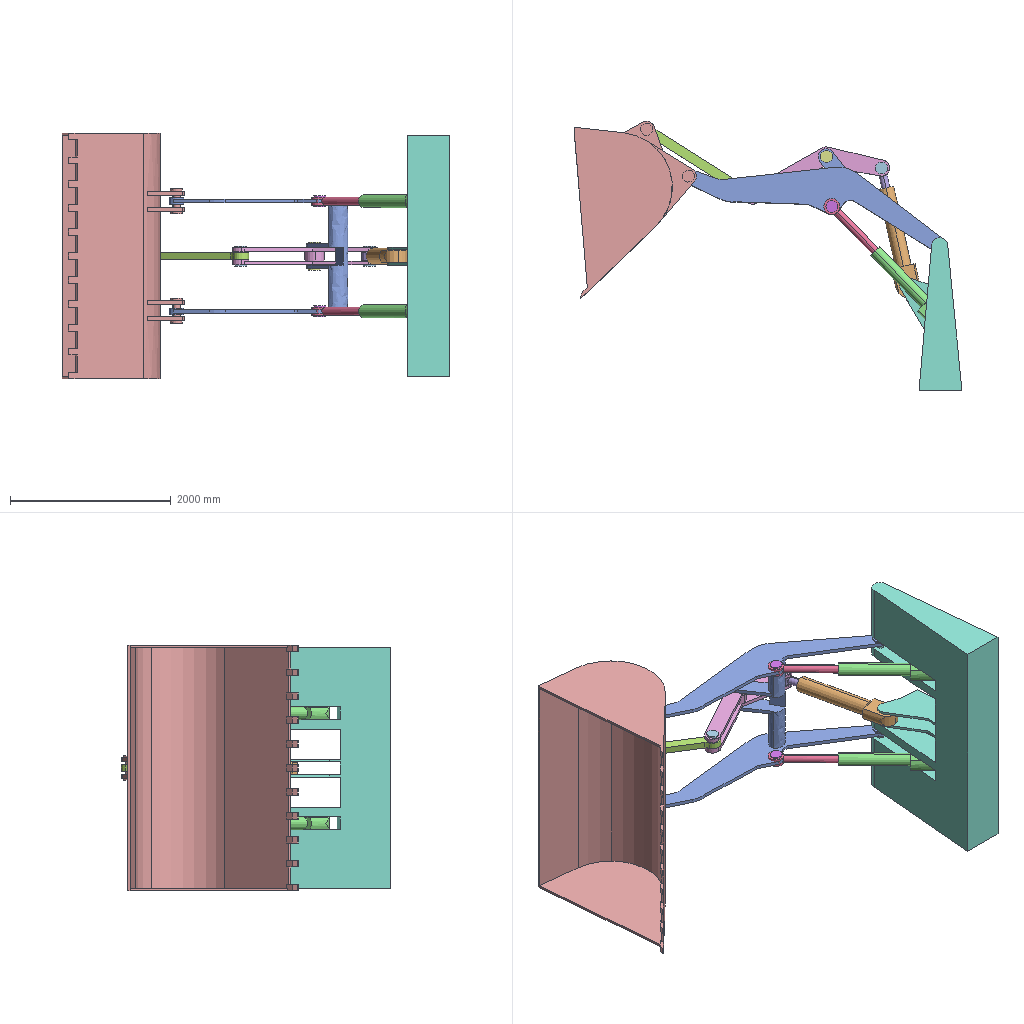Assembly | SolidWorks | 12 different items | 16 placed | box 4827 x 3349 x 3060 mm
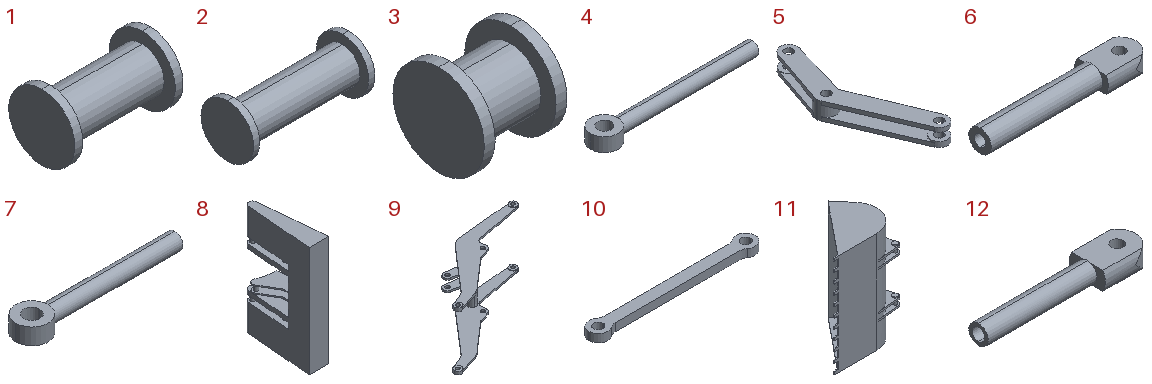Parts list (item | quantity | size | volume | features):
1 | x2 | 246 x 150 x 150 mm | 2285509 mm3 | features ICE 2, Extrusion 1
2 | x1 | 347 x 150 x 150 mm | 3078761 mm3 | features ICE 2, Extrusion 1
3 | x2 | 136 x 150 x 150 mm | 1421571 mm3 | features ICE 2, Extrusion 1
4 | x2 | 1182 x 200 x 100 mm | 10096773 mm3 | features Extrusion 1, ICE 1
5 | x1 | 614.266 x 1830 x 210 mm | 39335089 mm3 | features ICE 5, Extrusion 1
6 | x1 | 1400 x 300 x 200 mm | 38372929 mm3 | features ICE 3, Extrusion 1
7 | x1 | 982.338 x 200 x 100 mm | 8525978 mm3 | features Extrusion 1, ICE 1
8 | x1 | 773.621 x 1900 x 3000 mm | 1564577598 mm3 | features ICE 8, MirrorPattern 4, Extrusion 1
9 | x1 | 3058 x 1680 x 1452 mm | 154389748 mm3 | features ICE 8, MirrorPattern 2, Cut 1, Extrusion 1
10 | x1 | 1761 x 200 x 84 mm | 17816278 mm3 | features Extrusion 1
11 | x1 | 2144 x 1589 x 3060 mm | 438244984 mm3 | features ICE 11, Extrusion 1, LPattern 1, MirrorPattern 1
12 | x2 | 1300 x 300 x 160 mm | 25837974 mm3 | features ICE 3, Extrusion 1
Mates (type | each side: item.copy, entity, surface, feature):
Concentric | 11.1 face cylinder Boss-Extrude8 | 9.1 face cylinder Mirror2
DistanceDim | 9.1 face plane Mirror2 | 11.1 face plane Boss-Extrude5
Concentric | 9.1 face cylinder Boss-Extrude7 | 5.1 face cylinder Boss-Extrude1
DistanceDim | 5.1 face plane Boss-Extrude1 | 9.1 face plane Mirror1
Concentric | 11.1 face cylinder Boss-Extrude12 | 10.1 face cylinder Boss-Extrude1
DistanceDim | 10.1 face plane Boss-Extrude1 | 11.1 face plane Boss-Extrude7
Concentric | 10.1 face cylinder Boss-Extrude1 | 5.1 face cylinder Boss-Extrude1
Concentric | 9.1 face cylinder Mirror2 | 8.1 face cylinder Boss-Extrude3
DistanceDim | 8.1 face plane Cut-Extrude1 | 9.1 face plane Mirror2
Concentric | 6.1 face cylinder Boss-Extrude1 | 7.1 face cylinder Boss-Extrude1
Concentric | 5.1 face cylinder Boss-Extrude4 | 7.1 face cylinder Boss-Extrude2
DistanceDim | 7.1 face plane Boss-Extrude2 | 5.1 face plane Boss-Extrude3
Concentric | 8.1 face cylinder Boss-Extrude4 | 6.1 face cylinder Cut-Extrude3
Concentric | 8.1 face cylinder Boss-Extrude5 | 12.1 face cylinder Cut-Extrude3
DistanceDim | 12.1 face plane Boss-Extrude2 | 8.1 face plane Cut-Extrude1
Concentric | 12.1 face cylinder Boss-Extrude1 | 4.1 face cylinder Boss-Extrude1
Concentric | 9.1 face cylinder Mirror2 | 4.1 face cylinder Boss-Extrude2
Concentric | 3.1 face cylinder Boss-Extrude2 | 4.2 face cylinder Boss-Extrude2
Coincident | 4.2 face plane Boss-Extrude2 | 3.1 face plane Boss-Extrude1
Concentric | 9.1 face cylinder Mirror1 | 2.1 face cylinder Boss-Extrude2
Coincident | 9.1 face plane Mirror1 | 2.1 face plane Boss-Extrude3
Coincident | 5.1 face plane Boss-Extrude1 | 1.1 face plane Boss-Extrude1
Concentric | 5.1 face cylinder Boss-Extrude1 | 1.1 face cylinder Boss-Extrude2
Concentric | 5.1 face cylinder Boss-Extrude1 | 1.2 face cylinder Boss-Extrude2
Coincident | 5.1 face plane Boss-Extrude4 | 1.2 face plane Boss-Extrude3